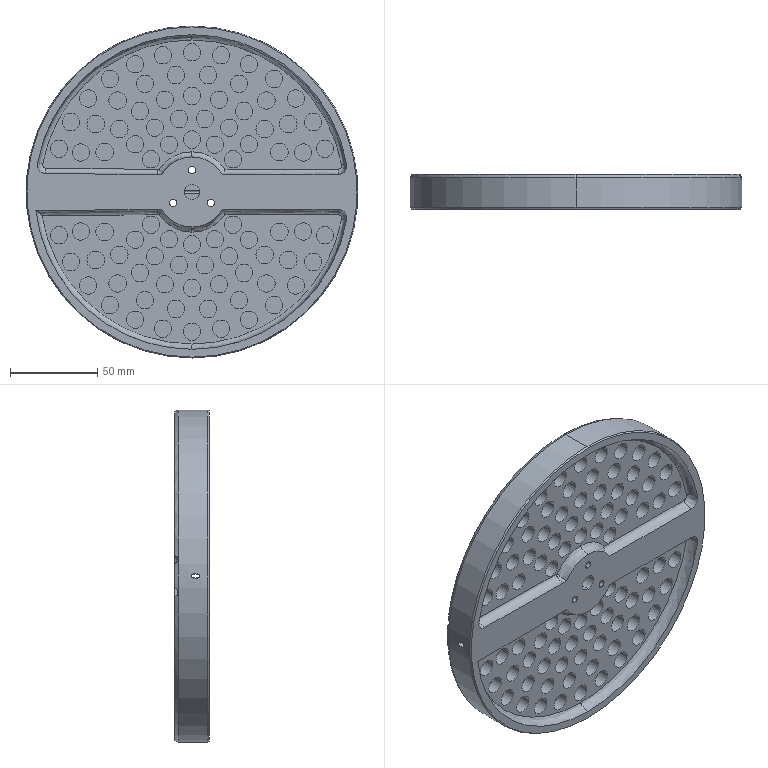Part | NX | features BREP 1 | 1 solid | 348 faces | box 190 x 20 x 190 mm | volume 260933 mm3 | cylinder 188 | plane 101 | spline 53 | cone 6 | commonest cylinder face diameters 10 x172 4.175 x6 3.722 x2 5.496 x2 9 x2 35.1 x2